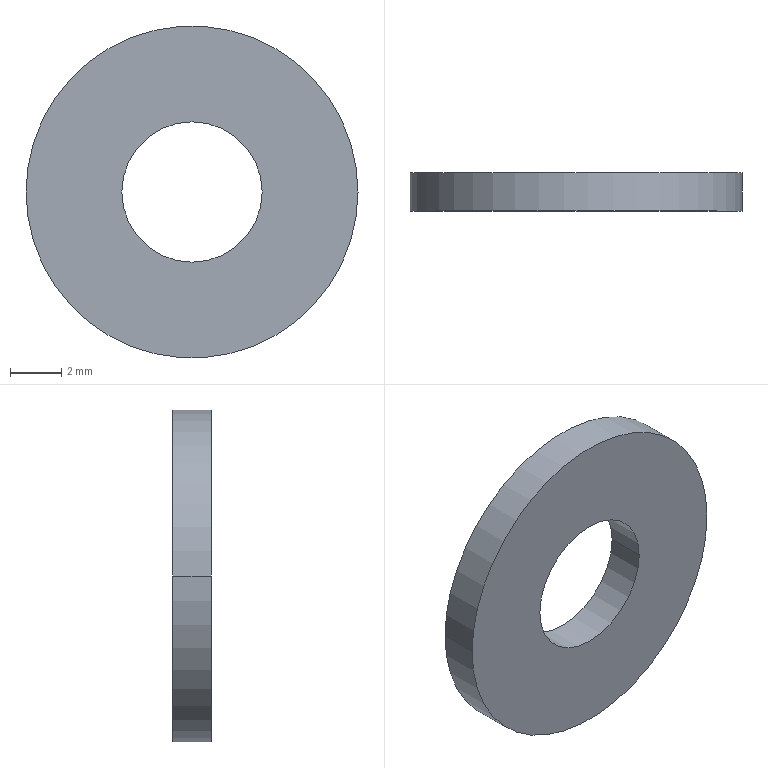Part | STEP file | TWSSS13-5.5-1.5-7 | 1 solid | 6 faces | box 13 x 1.5 x 13 mm | volume 163.461 mm3 | cylinder 4 | plane 2 | commonest cylinder face diameters 5.5 x2 13 x2
STEP:
#1=CARTESIAN_POINT('',(-2.75,0.,0.));
#2=VERTEX_POINT('',#1);
#3=CARTESIAN_POINT('',(2.75,0.,0.));
#4=VERTEX_POINT('',#3);
#5=CARTESIAN_POINT('',(0.,0.,0.));
#6=DIRECTION('',(0.,1.,0.));
#7=DIRECTION('',(1.,0.,0.));
#8=AXIS2_PLACEMENT_3D('',#5,#6,#7);
#9=CIRCLE('',#8,2.75);
#10=EDGE_CURVE('',#2,#4,#9,.T.);
#11=ORIENTED_EDGE('',*,*,#10,.F.);
#12=CARTESIAN_POINT('',(-2.75,1.5,0.));
#13=VERTEX_POINT('',#12);
#14=CARTESIAN_POINT('',(-2.75,0.,0.));
#15=DIRECTION('',(0.,1.,0.));
#16=VECTOR('',#15,1000.);
#17=LINE('',#14,#16);
#18=EDGE_CURVE('',#2,#13,#17,.T.);
#19=ORIENTED_EDGE('',*,*,#18,.T.);
#20=CARTESIAN_POINT('',(2.75,1.5,0.));
#21=VERTEX_POINT('',#20);
#22=CARTESIAN_POINT('',(0.,1.5,0.));
#23=DIRECTION('',(0.,-1.,0.));
#24=DIRECTION('',(-1.,0.,0.));
#25=AXIS2_PLACEMENT_3D('',#22,#23,#24);
#26=CIRCLE('',#25,2.75);
#27=EDGE_CURVE('',#21,#13,#26,.T.);
#28=ORIENTED_EDGE('',*,*,#27,.F.);
#29=CARTESIAN_POINT('',(2.75,0.,0.));
#30=DIRECTION('',(0.,1.,0.));
#31=VECTOR('',#30,1000.);
#32=LINE('',#29,#31);
#33=EDGE_CURVE('',#4,#21,#32,.T.);
#34=ORIENTED_EDGE('',*,*,#33,.F.);
#35=EDGE_LOOP('',(#11,#19,#28,#34));
#36=FACE_OUTER_BOUND('',#35,.T.);
#37=CARTESIAN_POINT('',(0.,0.,0.));
#38=DIRECTION('',(0.,1.,0.));
#39=DIRECTION('',(1.,0.,0.));
#40=AXIS2_PLACEMENT_3D('',#37,#38,#39);
#41=CYLINDRICAL_SURFACE('',#40,2.75);
#42=ADVANCED_FACE('',(#36),#41,.F.);
#43=CARTESIAN_POINT('',(6.5,0.,0.));
#44=VERTEX_POINT('',#43);
#45=CARTESIAN_POINT('',(-6.5,0.,0.));
#46=VERTEX_POINT('',#45);
#47=CARTESIAN_POINT('',(0.,0.,0.));
#48=DIRECTION('',(0.,1.,0.));
#49=DIRECTION('',(1.,0.,0.));
#50=AXIS2_PLACEMENT_3D('',#47,#48,#49);
#51=CIRCLE('',#50,6.5);
#52=EDGE_CURVE('',#44,#46,#51,.T.);
#53=ORIENTED_EDGE('',*,*,#52,.T.);
#54=CARTESIAN_POINT('',(-6.5,1.5,0.));
#55=VERTEX_POINT('',#54);
#56=CARTESIAN_POINT('',(-6.5,0.,0.));
#57=DIRECTION('',(0.,1.,0.));
#58=VECTOR('',#57,1000.);
#59=LINE('',#56,#58);
#60=EDGE_CURVE('',#46,#55,#59,.T.);
#61=ORIENTED_EDGE('',*,*,#60,.T.);
#62=CARTESIAN_POINT('',(6.5,1.5,0.));
#63=VERTEX_POINT('',#62);
#64=CARTESIAN_POINT('',(0.,1.5,0.));
#65=DIRECTION('',(0.,-1.,0.));
#66=DIRECTION('',(-1.,0.,0.));
#67=AXIS2_PLACEMENT_3D('',#64,#65,#66);
#68=CIRCLE('',#67,6.5);
#69=EDGE_CURVE('',#55,#63,#68,.T.);
#70=ORIENTED_EDGE('',*,*,#69,.T.);
#71=CARTESIAN_POINT('',(6.5,0.,0.));
#72=DIRECTION('',(0.,1.,0.));
#73=VECTOR('',#72,1000.);
#74=LINE('',#71,#73);
#75=EDGE_CURVE('',#44,#63,#74,.T.);
#76=ORIENTED_EDGE('',*,*,#75,.F.);
#77=EDGE_LOOP('',(#53,#61,#70,#76));
#78=FACE_OUTER_BOUND('',#77,.T.);
#79=CARTESIAN_POINT('',(0.,0.,0.));
#80=DIRECTION('',(0.,1.,0.));
#81=DIRECTION('',(1.,0.,0.));
#82=AXIS2_PLACEMENT_3D('',#79,#80,#81);
#83=CYLINDRICAL_SURFACE('',#82,6.5);
#84=ADVANCED_FACE('',(#78),#83,.T.);
#85=ORIENTED_EDGE('',*,*,#27,.T.);
#86=CARTESIAN_POINT('',(0.,1.5,0.));
#87=DIRECTION('',(0.,-1.,0.));
#88=DIRECTION('',(-1.,0.,0.));
#89=AXIS2_PLACEMENT_3D('',#86,#87,#88);
#90=CIRCLE('',#89,2.75);
#91=EDGE_CURVE('',#13,#21,#90,.T.);
#92=ORIENTED_EDGE('',*,*,#91,.T.);
#93=EDGE_LOOP('',(#85,#92));
#94=FACE_BOUND('',#93,.T.);
#95=CARTESIAN_POINT('',(0.,1.5,0.));
#96=DIRECTION('',(0.,-1.,0.));
#97=DIRECTION('',(-1.,0.,0.));
#98=AXIS2_PLACEMENT_3D('',#95,#96,#97);
#99=CIRCLE('',#98,6.5);
#100=EDGE_CURVE('',#63,#55,#99,.T.);
#101=ORIENTED_EDGE('',*,*,#100,.F.);
#102=ORIENTED_EDGE('',*,*,#69,.F.);
#103=EDGE_LOOP('',(#101,#102));
#104=FACE_OUTER_BOUND('',#103,.T.);
#105=CARTESIAN_POINT('',(0.,1.5,0.));
#106=DIRECTION('',(0.,1.,0.));
#107=DIRECTION('',(1.,0.,0.));
#108=AXIS2_PLACEMENT_3D('',#105,#106,#107);
#109=PLANE('',#108);
#110=ADVANCED_FACE('',(#94,#104),#109,.T.);
#111=CARTESIAN_POINT('',(0.,0.,0.));
#112=DIRECTION('',(0.,1.,0.));
#113=DIRECTION('',(1.,0.,0.));
#114=AXIS2_PLACEMENT_3D('',#111,#112,#113);
#115=CIRCLE('',#114,2.75);
#116=EDGE_CURVE('',#4,#2,#115,.T.);
#117=ORIENTED_EDGE('',*,*,#116,.T.);
#118=ORIENTED_EDGE('',*,*,#10,.T.);
#119=EDGE_LOOP('',(#117,#118));
#120=FACE_BOUND('',#119,.T.);
#121=ORIENTED_EDGE('',*,*,#52,.F.);
#122=CARTESIAN_POINT('',(0.,0.,0.));
#123=DIRECTION('',(0.,1.,0.));
#124=DIRECTION('',(1.,0.,0.));
#125=AXIS2_PLACEMENT_3D('',#122,#123,#124);
#126=CIRCLE('',#125,6.5);
#127=EDGE_CURVE('',#46,#44,#126,.T.);
#128=ORIENTED_EDGE('',*,*,#127,.F.);
#129=EDGE_LOOP('',(#121,#128));
#130=FACE_OUTER_BOUND('',#129,.T.);
#131=CARTESIAN_POINT('',(0.,0.,0.));
#132=DIRECTION('',(0.,-1.,0.));
#133=DIRECTION('',(-1.,0.,0.));
#134=AXIS2_PLACEMENT_3D('',#131,#132,#133);
#135=PLANE('',#134);
#136=ADVANCED_FACE('',(#120,#130),#135,.T.);
#137=ORIENTED_EDGE('',*,*,#60,.F.);
#138=ORIENTED_EDGE('',*,*,#127,.T.);
#139=ORIENTED_EDGE('',*,*,#75,.T.);
#140=ORIENTED_EDGE('',*,*,#100,.T.);
#141=EDGE_LOOP('',(#137,#138,#139,#140));
#142=FACE_OUTER_BOUND('',#141,.T.);
#143=CARTESIAN_POINT('',(0.,0.,0.));
#144=DIRECTION('',(0.,1.,0.));
#145=DIRECTION('',(1.,0.,0.));
#146=AXIS2_PLACEMENT_3D('',#143,#144,#145);
#147=CYLINDRICAL_SURFACE('',#146,6.5);
#148=ADVANCED_FACE('',(#142),#147,.T.);
#149=ORIENTED_EDGE('',*,*,#18,.F.);
#150=ORIENTED_EDGE('',*,*,#116,.F.);
#151=ORIENTED_EDGE('',*,*,#33,.T.);
#152=ORIENTED_EDGE('',*,*,#91,.F.);
#153=EDGE_LOOP('',(#149,#150,#151,#152));
#154=FACE_OUTER_BOUND('',#153,.T.);
#155=CARTESIAN_POINT('',(0.,0.,0.));
#156=DIRECTION('',(0.,1.,0.));
#157=DIRECTION('',(1.,0.,0.));
#158=AXIS2_PLACEMENT_3D('',#155,#156,#157);
#159=CYLINDRICAL_SURFACE('',#158,2.75);
#160=ADVANCED_FACE('',(#154),#159,.F.);
#161=CLOSED_SHELL('',(#42,#84,#110,#136,#148,#160));
#162=MANIFOLD_SOLID_BREP('',#161);
#163=CARTESIAN_POINT('',(0.,0.,0.));
#164=DIRECTION('',(0.,0.,1.));
#165=DIRECTION('',(1.,0.,0.));
#166=AXIS2_PLACEMENT_3D('',#163,#164,#165);
#167=(LENGTH_UNIT()NAMED_UNIT(*)SI_UNIT(.MILLI.,.METRE.));
#168=UNCERTAINTY_MEASURE_WITH_UNIT(LENGTH_MEASURE(0.00001),#167,'','');
#169=(NAMED_UNIT(*)PLANE_ANGLE_UNIT()SI_UNIT($,.RADIAN.));
#170=(NAMED_UNIT(*)SI_UNIT($,.STERADIAN.)SOLID_ANGLE_UNIT());
#171=(GEOMETRIC_REPRESENTATION_CONTEXT(3)GLOBAL_UNCERTAINTY_ASSIGNED_CONTEXT((#168))GLOBAL_UNIT_ASSIGNED_CONTEXT((#167,#169,#170))REPRESENTATION_CONTEXT('',''));
#172=ADVANCED_BREP_SHAPE_REPRESENTATION('',(#162,#166),#171);